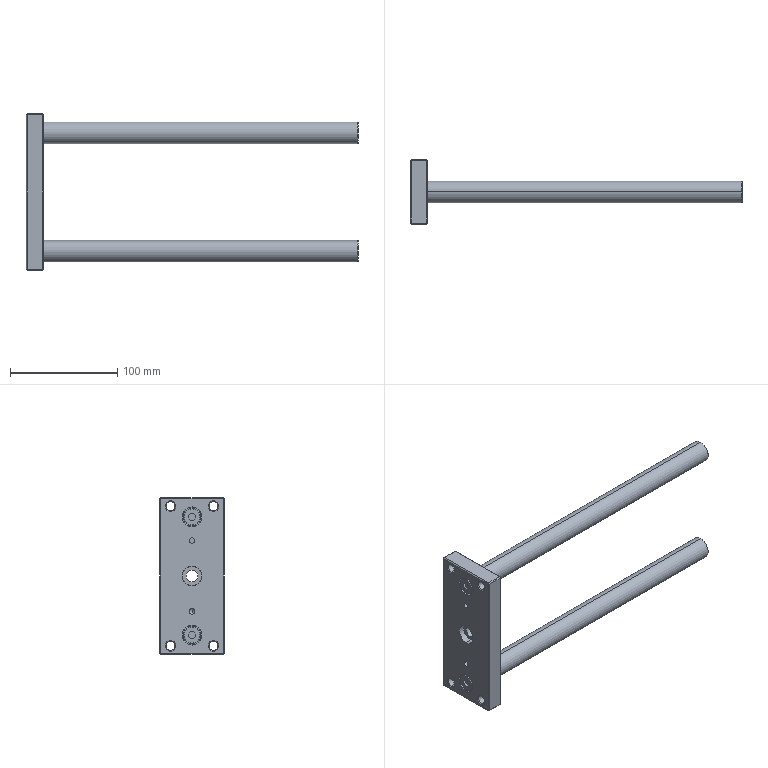Part | STEP file | TC_L_50x175_175fp | 1 solid | 107 faces | box 309 x 60 x 146 mm | volume 316571 mm3 | plane 44 | cylinder 31 | cone 28 | torus 4 | commonest cylinder face diameters 8.376 x8 5 x7 18 x6 16 x4 20 x4 11 x2